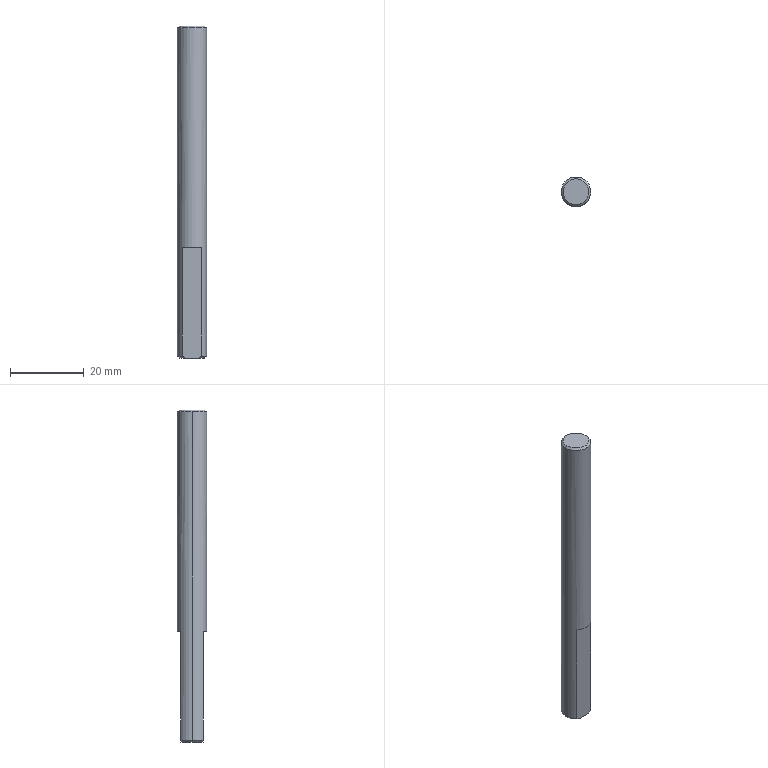Part | NX | features BREP 1 | 1 solid | 13 faces | box 8 x 8 x 90 mm | volume 4302 mm3 | plane 6 | cone 5 | cylinder 2 | commonest cylinder face diameters 8 x2
STEP:
#1=CARTESIAN_POINT('',(3.5,0.,90.));
#2=VERTEX_POINT('',#1);
#3=CARTESIAN_POINT('',(-3.5,0.,90.));
#4=VERTEX_POINT('',#3);
#5=CARTESIAN_POINT('',(0.,0.,90.));
#6=DIRECTION('',(0.,0.,1.));
#7=DIRECTION('',(1.,0.,0.));
#8=AXIS2_PLACEMENT_3D('',#5,#6,#7);
#9=CIRCLE('',#8,3.5);
#10=EDGE_CURVE('',#2,#4,#9,.T.);
#11=ORIENTED_EDGE('',*,*,#10,.F.);
#12=CARTESIAN_POINT('',(4.,0.,89.5));
#13=VERTEX_POINT('',#12);
#14=CARTESIAN_POINT('',(3.5,0.,90.));
#15=DIRECTION('',(0.7071,0.,-0.7071));
#16=VECTOR('',#15,1000.);
#17=LINE('',#14,#16);
#18=EDGE_CURVE('',#2,#13,#17,.T.);
#19=ORIENTED_EDGE('',*,*,#18,.T.);
#20=CARTESIAN_POINT('',(-4.,0.,89.5));
#21=VERTEX_POINT('',#20);
#22=CARTESIAN_POINT('',(0.,0.,89.5));
#23=DIRECTION('',(0.,0.,-1.));
#24=DIRECTION('',(1.,0.,0.));
#25=AXIS2_PLACEMENT_3D('',#22,#23,#24);
#26=CIRCLE('',#25,4.);
#27=EDGE_CURVE('',#21,#13,#26,.T.);
#28=ORIENTED_EDGE('',*,*,#27,.F.);
#29=CARTESIAN_POINT('',(-3.5,0.,90.));
#30=DIRECTION('',(-0.7071,0.,-0.7071));
#31=VECTOR('',#30,1000.);
#32=LINE('',#29,#31);
#33=EDGE_CURVE('',#4,#21,#32,.T.);
#34=ORIENTED_EDGE('',*,*,#33,.F.);
#35=EDGE_LOOP('',(#11,#19,#28,#34));
#36=FACE_BOUND('',#35,.T.);
#37=CARTESIAN_POINT('',(0.,0.,90.));
#38=DIRECTION('',(0.,0.,-1.));
#39=DIRECTION('',(-1.,0.,0.));
#40=AXIS2_PLACEMENT_3D('',#37,#38,#39);
#41=CONICAL_SURFACE('',#40,3.5,0.7854);
#42=ADVANCED_FACE('',(#36),#41,.T.);
#43=CARTESIAN_POINT('',(3.5,0.,0.));
#44=VERTEX_POINT('',#43);
#45=CARTESIAN_POINT('',(1.803,-3.,0.));
#46=VERTEX_POINT('',#45);
#47=CARTESIAN_POINT('',(0.,0.,0.));
#48=DIRECTION('',(0.,0.,-1.));
#49=DIRECTION('',(1.,0.,0.));
#50=AXIS2_PLACEMENT_3D('',#47,#48,#49);
#51=CIRCLE('',#50,3.5);
#52=EDGE_CURVE('',#44,#46,#51,.T.);
#53=ORIENTED_EDGE('',*,*,#52,.F.);
#54=CARTESIAN_POINT('',(4.,0.,0.5));
#55=VERTEX_POINT('',#54);
#56=CARTESIAN_POINT('',(4.,0.,0.5));
#57=DIRECTION('',(0.7071,0.,0.7071));
#58=VECTOR('',#57,1000.);
#59=LINE('',#56,#58);
#60=EDGE_CURVE('',#44,#55,#59,.T.);
#61=ORIENTED_EDGE('',*,*,#60,.T.);
#62=CARTESIAN_POINT('',(2.646,-3.,0.5));
#63=VERTEX_POINT('',#62);
#64=CARTESIAN_POINT('',(0.,0.,0.5));
#65=DIRECTION('',(0.,0.,1.));
#66=DIRECTION('',(1.,0.,0.));
#67=AXIS2_PLACEMENT_3D('',#64,#65,#66);
#68=CIRCLE('',#67,4.);
#69=EDGE_CURVE('',#63,#55,#68,.T.);
#70=ORIENTED_EDGE('',*,*,#69,.F.);
#71=CARTESIAN_POINT('',(1.803,-3.,0.));
#72=CARTESIAN_POINT('',(2.065,-3.,0.1351));
#73=CARTESIAN_POINT('',(2.346,-3.,0.3018));
#74=CARTESIAN_POINT('',(2.646,-3.,0.5));
#75=B_SPLINE_CURVE_WITH_KNOTS('',3,(#71,#72,#73,#74),.UNSPECIFIED.,.F.,.F.,(4,4),(0.,1.),.UNSPECIFIED.);
#76=EDGE_CURVE('',#63,#46,#75,.F.);
#77=ORIENTED_EDGE('',*,*,#76,.T.);
#78=EDGE_LOOP('',(#53,#61,#70,#77));
#79=FACE_BOUND('',#78,.T.);
#80=CARTESIAN_POINT('',(0.,0.,0.5));
#81=DIRECTION('',(0.,0.,1.));
#82=DIRECTION('',(1.,0.,0.));
#83=AXIS2_PLACEMENT_3D('',#80,#81,#82);
#84=CONICAL_SURFACE('',#83,4.,0.7854);
#85=ADVANCED_FACE('',(#79),#84,.T.);
#86=ORIENTED_EDGE('',*,*,#27,.T.);
#87=CARTESIAN_POINT('',(4.,0.,90.));
#88=DIRECTION('',(0.,0.,-1.));
#89=VECTOR('',#88,1000.);
#90=LINE('',#87,#89);
#91=EDGE_CURVE('',#13,#55,#90,.T.);
#92=ORIENTED_EDGE('',*,*,#91,.T.);
#93=CARTESIAN_POINT('',(2.646,3.,0.5));
#94=VERTEX_POINT('',#93);
#95=CARTESIAN_POINT('',(0.,0.,0.5));
#96=DIRECTION('',(0.,0.,1.));
#97=DIRECTION('',(1.,0.,0.));
#98=AXIS2_PLACEMENT_3D('',#95,#96,#97);
#99=CIRCLE('',#98,4.);
#100=EDGE_CURVE('',#55,#94,#99,.T.);
#101=ORIENTED_EDGE('',*,*,#100,.T.);
#102=CARTESIAN_POINT('',(2.646,3.,30.));
#103=VERTEX_POINT('',#102);
#104=CARTESIAN_POINT('',(2.646,3.,90.));
#105=DIRECTION('',(0.,0.,-1.));
#106=VECTOR('',#105,1000.);
#107=LINE('',#104,#106);
#108=EDGE_CURVE('',#103,#94,#107,.T.);
#109=ORIENTED_EDGE('',*,*,#108,.F.);
#110=CARTESIAN_POINT('',(-2.646,3.,30.));
#111=VERTEX_POINT('',#110);
#112=CARTESIAN_POINT('',(0.,0.,30.));
#113=DIRECTION('',(0.,0.,-1.));
#114=DIRECTION('',(-1.,0.,0.));
#115=AXIS2_PLACEMENT_3D('',#112,#113,#114);
#116=CIRCLE('',#115,4.);
#117=EDGE_CURVE('',#111,#103,#116,.T.);
#118=ORIENTED_EDGE('',*,*,#117,.F.);
#119=CARTESIAN_POINT('',(-2.646,3.,0.5));
#120=VERTEX_POINT('',#119);
#121=CARTESIAN_POINT('',(-2.646,3.,90.));
#122=DIRECTION('',(0.,0.,1.));
#123=VECTOR('',#122,1000.);
#124=LINE('',#121,#123);
#125=EDGE_CURVE('',#120,#111,#124,.T.);
#126=ORIENTED_EDGE('',*,*,#125,.F.);
#127=CARTESIAN_POINT('',(-4.,0.,0.5));
#128=VERTEX_POINT('',#127);
#129=CARTESIAN_POINT('',(0.,0.,0.5));
#130=DIRECTION('',(0.,0.,1.));
#131=DIRECTION('',(1.,0.,0.));
#132=AXIS2_PLACEMENT_3D('',#129,#130,#131);
#133=CIRCLE('',#132,4.);
#134=EDGE_CURVE('',#120,#128,#133,.T.);
#135=ORIENTED_EDGE('',*,*,#134,.T.);
#136=CARTESIAN_POINT('',(-4.,0.,90.));
#137=DIRECTION('',(0.,0.,-1.));
#138=VECTOR('',#137,1000.);
#139=LINE('',#136,#138);
#140=EDGE_CURVE('',#21,#128,#139,.T.);
#141=ORIENTED_EDGE('',*,*,#140,.F.);
#142=EDGE_LOOP('',(#86,#92,#101,#109,#118,#126,#135,#141));
#143=FACE_BOUND('',#142,.T.);
#144=CARTESIAN_POINT('',(0.,0.,90.));
#145=DIRECTION('',(0.,0.,-1.));
#146=DIRECTION('',(-1.,0.,0.));
#147=AXIS2_PLACEMENT_3D('',#144,#145,#146);
#148=CYLINDRICAL_SURFACE('',#147,4.);
#149=ADVANCED_FACE('',(#143),#148,.T.);
#150=ORIENTED_EDGE('',*,*,#91,.F.);
#151=CARTESIAN_POINT('',(0.,0.,89.5));
#152=DIRECTION('',(0.,0.,-1.));
#153=DIRECTION('',(1.,0.,0.));
#154=AXIS2_PLACEMENT_3D('',#151,#152,#153);
#155=CIRCLE('',#154,4.);
#156=EDGE_CURVE('',#13,#21,#155,.T.);
#157=ORIENTED_EDGE('',*,*,#156,.T.);
#158=ORIENTED_EDGE('',*,*,#140,.T.);
#159=CARTESIAN_POINT('',(-2.646,-3.,0.5));
#160=VERTEX_POINT('',#159);
#161=CARTESIAN_POINT('',(0.,0.,0.5));
#162=DIRECTION('',(0.,0.,1.));
#163=DIRECTION('',(1.,0.,0.));
#164=AXIS2_PLACEMENT_3D('',#161,#162,#163);
#165=CIRCLE('',#164,4.);
#166=EDGE_CURVE('',#128,#160,#165,.T.);
#167=ORIENTED_EDGE('',*,*,#166,.T.);
#168=CARTESIAN_POINT('',(-2.646,-3.,30.));
#169=VERTEX_POINT('',#168);
#170=CARTESIAN_POINT('',(-2.646,-3.,90.));
#171=DIRECTION('',(0.,0.,-1.));
#172=VECTOR('',#171,1000.);
#173=LINE('',#170,#172);
#174=EDGE_CURVE('',#169,#160,#173,.T.);
#175=ORIENTED_EDGE('',*,*,#174,.F.);
#176=CARTESIAN_POINT('',(2.646,-3.,30.));
#177=VERTEX_POINT('',#176);
#178=CARTESIAN_POINT('',(0.,0.,30.));
#179=DIRECTION('',(0.,0.,-1.));
#180=DIRECTION('',(-1.,0.,0.));
#181=AXIS2_PLACEMENT_3D('',#178,#179,#180);
#182=CIRCLE('',#181,4.);
#183=EDGE_CURVE('',#177,#169,#182,.T.);
#184=ORIENTED_EDGE('',*,*,#183,.F.);
#185=CARTESIAN_POINT('',(2.646,-3.,90.));
#186=DIRECTION('',(0.,0.,1.));
#187=VECTOR('',#186,1000.);
#188=LINE('',#185,#187);
#189=EDGE_CURVE('',#63,#177,#188,.T.);
#190=ORIENTED_EDGE('',*,*,#189,.F.);
#191=ORIENTED_EDGE('',*,*,#69,.T.);
#192=EDGE_LOOP('',(#150,#157,#158,#167,#175,#184,#190,#191));
#193=FACE_BOUND('',#192,.T.);
#194=CARTESIAN_POINT('',(0.,0.,90.));
#195=DIRECTION('',(0.,0.,-1.));
#196=DIRECTION('',(-1.,0.,0.));
#197=AXIS2_PLACEMENT_3D('',#194,#195,#196);
#198=CYLINDRICAL_SURFACE('',#197,4.);
#199=ADVANCED_FACE('',(#193),#198,.T.);
#200=CARTESIAN_POINT('',(-1.803,-3.,0.));
#201=VERTEX_POINT('',#200);
#202=CARTESIAN_POINT('',(5.343,-3.,0.));
#203=DIRECTION('',(-1.,0.,0.));
#204=VECTOR('',#203,1000.);
#205=LINE('',#202,#204);
#206=EDGE_CURVE('',#46,#201,#205,.T.);
#207=ORIENTED_EDGE('',*,*,#206,.T.);
#208=CARTESIAN_POINT('',(-1.803,3.,0.));
#209=VERTEX_POINT('',#208);
#210=CARTESIAN_POINT('',(0.,0.,0.));
#211=DIRECTION('',(0.,0.,-1.));
#212=DIRECTION('',(1.,0.,0.));
#213=AXIS2_PLACEMENT_3D('',#210,#211,#212);
#214=CIRCLE('',#213,3.5);
#215=EDGE_CURVE('',#201,#209,#214,.T.);
#216=ORIENTED_EDGE('',*,*,#215,.T.);
#217=CARTESIAN_POINT('',(1.803,3.,0.));
#218=VERTEX_POINT('',#217);
#219=CARTESIAN_POINT('',(5.343,3.,0.));
#220=DIRECTION('',(1.,0.,0.));
#221=VECTOR('',#220,1000.);
#222=LINE('',#219,#221);
#223=EDGE_CURVE('',#209,#218,#222,.T.);
#224=ORIENTED_EDGE('',*,*,#223,.T.);
#225=CARTESIAN_POINT('',(0.,0.,0.));
#226=DIRECTION('',(0.,0.,-1.));
#227=DIRECTION('',(1.,0.,0.));
#228=AXIS2_PLACEMENT_3D('',#225,#226,#227);
#229=CIRCLE('',#228,3.5);
#230=EDGE_CURVE('',#218,#44,#229,.T.);
#231=ORIENTED_EDGE('',*,*,#230,.T.);
#232=ORIENTED_EDGE('',*,*,#52,.T.);
#233=EDGE_LOOP('',(#207,#216,#224,#231,#232));
#234=FACE_BOUND('',#233,.T.);
#235=CARTESIAN_POINT('',(0.,0.,0.));
#236=DIRECTION('',(0.,0.,1.));
#237=DIRECTION('',(1.,0.,0.));
#238=AXIS2_PLACEMENT_3D('',#235,#236,#237);
#239=PLANE('',#238);
#240=ADVANCED_FACE('',(#234),#239,.F.);
#241=ORIENTED_EDGE('',*,*,#60,.F.);
#242=ORIENTED_EDGE('',*,*,#230,.F.);
#243=CARTESIAN_POINT('',(2.646,3.,0.5));
#244=CARTESIAN_POINT('',(2.346,3.,0.3018));
#245=CARTESIAN_POINT('',(2.065,3.,0.1351));
#246=CARTESIAN_POINT('',(1.803,3.,0.));
#247=B_SPLINE_CURVE_WITH_KNOTS('',3,(#243,#244,#245,#246),.UNSPECIFIED.,.F.,.F.,(4,4),(0.,1.),.UNSPECIFIED.);
#248=EDGE_CURVE('',#218,#94,#247,.F.);
#249=ORIENTED_EDGE('',*,*,#248,.T.);
#250=ORIENTED_EDGE('',*,*,#100,.F.);
#251=EDGE_LOOP('',(#241,#242,#249,#250));
#252=FACE_BOUND('',#251,.T.);
#253=CARTESIAN_POINT('',(0.,0.,0.5));
#254=DIRECTION('',(0.,0.,1.));
#255=DIRECTION('',(1.,0.,0.));
#256=AXIS2_PLACEMENT_3D('',#253,#254,#255);
#257=CONICAL_SURFACE('',#256,4.,0.7854);
#258=ADVANCED_FACE('',(#252),#257,.T.);
#259=ORIENTED_EDGE('',*,*,#215,.F.);
#260=CARTESIAN_POINT('',(-2.646,-3.,0.5));
#261=CARTESIAN_POINT('',(-2.346,-3.,0.3018));
#262=CARTESIAN_POINT('',(-2.065,-3.,0.1351));
#263=CARTESIAN_POINT('',(-1.803,-3.,0.));
#264=B_SPLINE_CURVE_WITH_KNOTS('',3,(#260,#261,#262,#263),.UNSPECIFIED.,.F.,.F.,(4,4),(0.,1.),.UNSPECIFIED.);
#265=EDGE_CURVE('',#201,#160,#264,.F.);
#266=ORIENTED_EDGE('',*,*,#265,.T.);
#267=ORIENTED_EDGE('',*,*,#166,.F.);
#268=ORIENTED_EDGE('',*,*,#134,.F.);
#269=CARTESIAN_POINT('',(-1.803,3.,0.));
#270=CARTESIAN_POINT('',(-2.065,3.,0.1351));
#271=CARTESIAN_POINT('',(-2.346,3.,0.3018));
#272=CARTESIAN_POINT('',(-2.646,3.,0.5));
#273=B_SPLINE_CURVE_WITH_KNOTS('',3,(#269,#270,#271,#272),.UNSPECIFIED.,.F.,.F.,(4,4),(0.,1.),.UNSPECIFIED.);
#274=EDGE_CURVE('',#120,#209,#273,.F.);
#275=ORIENTED_EDGE('',*,*,#274,.T.);
#276=EDGE_LOOP('',(#259,#266,#267,#268,#275));
#277=FACE_BOUND('',#276,.T.);
#278=CARTESIAN_POINT('',(0.,0.,0.5));
#279=DIRECTION('',(0.,0.,1.));
#280=DIRECTION('',(1.,0.,0.));
#281=AXIS2_PLACEMENT_3D('',#278,#279,#280);
#282=CONICAL_SURFACE('',#281,4.,0.7854);
#283=ADVANCED_FACE('',(#277),#282,.T.);
#284=CARTESIAN_POINT('',(0.,0.,90.));
#285=DIRECTION('',(0.,0.,1.));
#286=DIRECTION('',(1.,0.,0.));
#287=AXIS2_PLACEMENT_3D('',#284,#285,#286);
#288=CIRCLE('',#287,3.5);
#289=EDGE_CURVE('',#4,#2,#288,.T.);
#290=ORIENTED_EDGE('',*,*,#289,.T.);
#291=ORIENTED_EDGE('',*,*,#10,.T.);
#292=EDGE_LOOP('',(#290,#291));
#293=FACE_BOUND('',#292,.T.);
#294=CARTESIAN_POINT('',(0.,0.,90.));
#295=DIRECTION('',(0.,0.,1.));
#296=DIRECTION('',(1.,0.,0.));
#297=AXIS2_PLACEMENT_3D('',#294,#295,#296);
#298=PLANE('',#297);
#299=ADVANCED_FACE('',(#293),#298,.T.);
#300=ORIENTED_EDGE('',*,*,#18,.F.);
#301=ORIENTED_EDGE('',*,*,#289,.F.);
#302=ORIENTED_EDGE('',*,*,#33,.T.);
#303=ORIENTED_EDGE('',*,*,#156,.F.);
#304=EDGE_LOOP('',(#300,#301,#302,#303));
#305=FACE_BOUND('',#304,.T.);
#306=CARTESIAN_POINT('',(0.,0.,90.));
#307=DIRECTION('',(0.,0.,-1.));
#308=DIRECTION('',(-1.,0.,0.));
#309=AXIS2_PLACEMENT_3D('',#306,#307,#308);
#310=CONICAL_SURFACE('',#309,3.5,0.7854);
#311=ADVANCED_FACE('',(#305),#310,.T.);
#312=ORIENTED_EDGE('',*,*,#125,.T.);
#313=CARTESIAN_POINT('',(5.343,3.,30.));
#314=DIRECTION('',(1.,0.,0.));
#315=VECTOR('',#314,1000.);
#316=LINE('',#313,#315);
#317=EDGE_CURVE('',#111,#103,#316,.T.);
#318=ORIENTED_EDGE('',*,*,#317,.T.);
#319=ORIENTED_EDGE('',*,*,#108,.T.);
#320=ORIENTED_EDGE('',*,*,#248,.F.);
#321=ORIENTED_EDGE('',*,*,#223,.F.);
#322=ORIENTED_EDGE('',*,*,#274,.F.);
#323=EDGE_LOOP('',(#312,#318,#319,#320,#321,#322));
#324=FACE_BOUND('',#323,.T.);
#325=CARTESIAN_POINT('',(5.343,3.,30.));
#326=DIRECTION('',(0.,1.,0.));
#327=DIRECTION('',(1.,0.,0.));
#328=AXIS2_PLACEMENT_3D('',#325,#326,#327);
#329=PLANE('',#328);
#330=ADVANCED_FACE('',(#324),#329,.T.);
#331=ORIENTED_EDGE('',*,*,#117,.T.);
#332=ORIENTED_EDGE('',*,*,#317,.F.);
#333=EDGE_LOOP('',(#331,#332));
#334=FACE_BOUND('',#333,.T.);
#335=CARTESIAN_POINT('',(0.,0.,30.));
#336=DIRECTION('',(0.,0.,-1.));
#337=DIRECTION('',(0.,-1.,0.));
#338=AXIS2_PLACEMENT_3D('',#335,#336,#337);
#339=PLANE('',#338);
#340=ADVANCED_FACE('',(#334),#339,.T.);
#341=ORIENTED_EDGE('',*,*,#183,.T.);
#342=CARTESIAN_POINT('',(5.343,-3.,30.));
#343=DIRECTION('',(-1.,0.,0.));
#344=VECTOR('',#343,1000.);
#345=LINE('',#342,#344);
#346=EDGE_CURVE('',#177,#169,#345,.T.);
#347=ORIENTED_EDGE('',*,*,#346,.F.);
#348=EDGE_LOOP('',(#341,#347));
#349=FACE_BOUND('',#348,.T.);
#350=CARTESIAN_POINT('',(0.,0.,30.));
#351=DIRECTION('',(0.,0.,-1.));
#352=DIRECTION('',(0.,-1.,0.));
#353=AXIS2_PLACEMENT_3D('',#350,#351,#352);
#354=PLANE('',#353);
#355=ADVANCED_FACE('',(#349),#354,.T.);
#356=ORIENTED_EDGE('',*,*,#189,.T.);
#357=ORIENTED_EDGE('',*,*,#346,.T.);
#358=ORIENTED_EDGE('',*,*,#174,.T.);
#359=ORIENTED_EDGE('',*,*,#265,.F.);
#360=ORIENTED_EDGE('',*,*,#206,.F.);
#361=ORIENTED_EDGE('',*,*,#76,.F.);
#362=EDGE_LOOP('',(#356,#357,#358,#359,#360,#361));
#363=FACE_BOUND('',#362,.T.);
#364=CARTESIAN_POINT('',(5.343,-3.,30.));
#365=DIRECTION('',(0.,-1.,0.));
#366=DIRECTION('',(0.,0.,-1.));
#367=AXIS2_PLACEMENT_3D('',#364,#365,#366);
#368=PLANE('',#367);
#369=ADVANCED_FACE('',(#363),#368,.T.);
#370=CLOSED_SHELL('',(#42,#85,#149,#199,#240,#258,#283,#299,#311,#330,#340,#355,#369));
#371=MANIFOLD_SOLID_BREP('',#370);
#372=(LENGTH_UNIT()NAMED_UNIT(*)SI_UNIT(.MILLI.,.METRE.));
#373=UNCERTAINTY_MEASURE_WITH_UNIT(LENGTH_MEASURE(0.0508),#372,'','');
#374=(NAMED_UNIT(*)PLANE_ANGLE_UNIT()SI_UNIT($,.RADIAN.));
#375=(NAMED_UNIT(*)SI_UNIT($,.STERADIAN.)SOLID_ANGLE_UNIT());
#376=(GEOMETRIC_REPRESENTATION_CONTEXT(3)GLOBAL_UNCERTAINTY_ASSIGNED_CONTEXT((#373))GLOBAL_UNIT_ASSIGNED_CONTEXT((#372,#374,#375))REPRESENTATION_CONTEXT('',''));
#377=ADVANCED_BREP_SHAPE_REPRESENTATION('',(#371),#376);